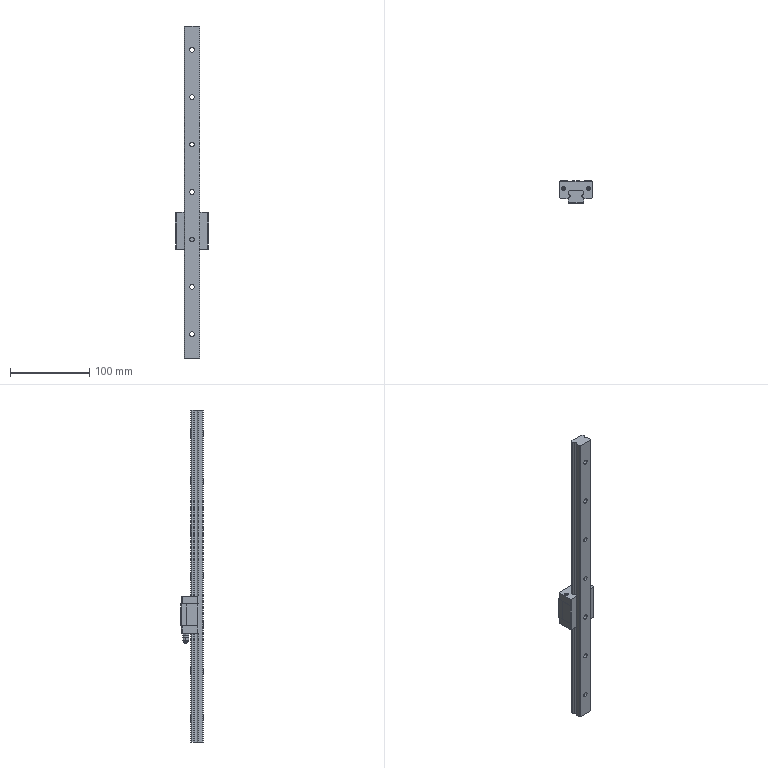Part | SolidWorks | 2 solids | 225 faces | box 42 x 28 x 420 mm | volume 150094 mm3 | plane 118 | cylinder 74 | cone 32 | torus 1 | commonest cylinder face diameters 3.08 x16 6 x14 9.5 x14 4.4 x8 4.8 x8 3 x4